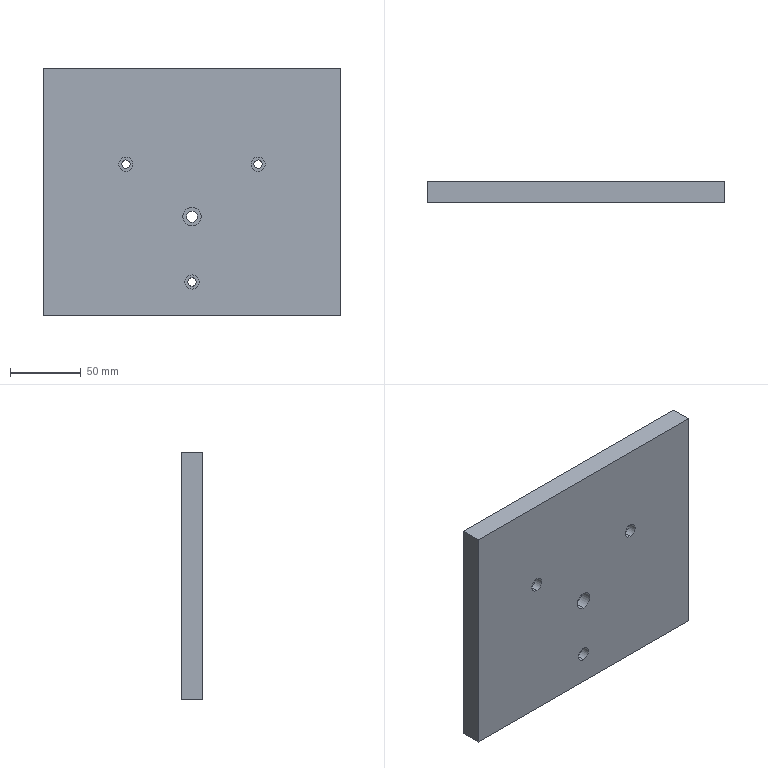Part | SolidWorks | features Cut 4, 3DProfileFeature 2, HoleWzd 2, Extrusion 1 | 1 solid | 46 faces | box 210 x 15 x 175 mm | volume 546137 mm3 | cylinder 26 | cone 10 | plane 10 | commonest cylinder face diameters 5 x10 6 x6 10 x6 8 x2 13 x2
STEP:
#1=CARTESIAN_POINT('',(0.,15.,-21.5));
#2=VERTEX_POINT('',#1);
#3=CARTESIAN_POINT('',(0.,15.,-13.5));
#4=VERTEX_POINT('',#3);
#5=CARTESIAN_POINT('',(0.,15.,-17.5));
#6=DIRECTION('',(0.,1.,0.));
#7=DIRECTION('',(0.,0.,-1.));
#8=AXIS2_PLACEMENT_3D('',#5,#6,#7);
#9=CIRCLE('',#8,4.);
#10=EDGE_CURVE('',#2,#4,#9,.T.);
#11=ORIENTED_EDGE('',*,*,#10,.T.);
#12=CARTESIAN_POINT('',(0.,8.,-13.5));
#13=VERTEX_POINT('',#12);
#14=CARTESIAN_POINT('',(0.,15.001,-13.5));
#15=DIRECTION('',(0.,-1.,0.));
#16=VECTOR('',#15,1000.);
#17=LINE('',#14,#16);
#18=EDGE_CURVE('',#4,#13,#17,.T.);
#19=ORIENTED_EDGE('',*,*,#18,.T.);
#20=CARTESIAN_POINT('',(0.,8.,-21.5));
#21=VERTEX_POINT('',#20);
#22=CARTESIAN_POINT('',(0.,8.,-17.5));
#23=DIRECTION('',(0.,1.,0.));
#24=DIRECTION('',(0.,0.,-1.));
#25=AXIS2_PLACEMENT_3D('',#22,#23,#24);
#26=CIRCLE('',#25,4.);
#27=EDGE_CURVE('',#21,#13,#26,.T.);
#28=ORIENTED_EDGE('',*,*,#27,.F.);
#29=CARTESIAN_POINT('',(0.,15.001,-21.5));
#30=DIRECTION('',(0.,-1.,0.));
#31=VECTOR('',#30,1000.);
#32=LINE('',#29,#31);
#33=EDGE_CURVE('',#2,#21,#32,.T.);
#34=ORIENTED_EDGE('',*,*,#33,.F.);
#35=EDGE_LOOP('',(#11,#19,#28,#34));
#36=FACE_OUTER_BOUND('',#35,.T.);
#37=CARTESIAN_POINT('',(0.,15.001,-17.5));
#38=DIRECTION('',(0.,-1.,0.));
#39=DIRECTION('',(0.,0.,-1.));
#40=AXIS2_PLACEMENT_3D('',#37,#38,#39);
#41=CYLINDRICAL_SURFACE('',#40,4.);
#42=ADVANCED_FACE('',(#36),#41,.F.);
#43=CARTESIAN_POINT('',(0.,8.,-11.));
#44=VERTEX_POINT('',#43);
#45=CARTESIAN_POINT('',(0.,8.,-24.));
#46=VERTEX_POINT('',#45);
#47=CARTESIAN_POINT('',(0.,8.,-17.5));
#48=DIRECTION('',(0.,-1.,0.));
#49=DIRECTION('',(0.,0.,-1.));
#50=AXIS2_PLACEMENT_3D('',#47,#48,#49);
#51=CIRCLE('',#50,6.5);
#52=EDGE_CURVE('',#44,#46,#51,.T.);
#53=ORIENTED_EDGE('',*,*,#52,.F.);
#54=CARTESIAN_POINT('',(0.,0.,-11.));
#55=VERTEX_POINT('',#54);
#56=CARTESIAN_POINT('',(0.,8.,-11.));
#57=DIRECTION('',(0.,-1.,0.));
#58=VECTOR('',#57,1000.);
#59=LINE('',#56,#58);
#60=EDGE_CURVE('',#44,#55,#59,.T.);
#61=ORIENTED_EDGE('',*,*,#60,.T.);
#62=CARTESIAN_POINT('',(0.,0.,-24.));
#63=VERTEX_POINT('',#62);
#64=CARTESIAN_POINT('',(0.,0.,-17.5));
#65=DIRECTION('',(0.,-1.,0.));
#66=DIRECTION('',(0.,0.,-1.));
#67=AXIS2_PLACEMENT_3D('',#64,#65,#66);
#68=CIRCLE('',#67,6.5);
#69=EDGE_CURVE('',#55,#63,#68,.T.);
#70=ORIENTED_EDGE('',*,*,#69,.T.);
#71=CARTESIAN_POINT('',(0.,8.,-24.));
#72=DIRECTION('',(0.,-1.,0.));
#73=VECTOR('',#72,1000.);
#74=LINE('',#71,#73);
#75=EDGE_CURVE('',#46,#63,#74,.T.);
#76=ORIENTED_EDGE('',*,*,#75,.F.);
#77=EDGE_LOOP('',(#53,#61,#70,#76));
#78=FACE_OUTER_BOUND('',#77,.T.);
#79=CARTESIAN_POINT('',(0.,8.,-17.5));
#80=DIRECTION('',(0.,-1.,0.));
#81=DIRECTION('',(0.,0.,-1.));
#82=AXIS2_PLACEMENT_3D('',#79,#80,#81);
#83=CYLINDRICAL_SURFACE('',#82,6.5);
#84=ADVANCED_FACE('',(#78),#83,.F.);
#85=CARTESIAN_POINT('',(82.5,7.5,-72.5));
#86=VERTEX_POINT('',#85);
#87=CARTESIAN_POINT('',(77.5,7.5,-72.5));
#88=VERTEX_POINT('',#87);
#89=CARTESIAN_POINT('',(80.,7.5,-72.5));
#90=DIRECTION('',(0.,0.,-1.));
#91=DIRECTION('',(-1.,0.,0.));
#92=AXIS2_PLACEMENT_3D('',#89,#90,#91);
#93=CIRCLE('',#92,2.5);
#94=EDGE_CURVE('',#86,#88,#93,.T.);
#95=ORIENTED_EDGE('',*,*,#94,.F.);
#96=CARTESIAN_POINT('',(82.5,7.5,-87.5));
#97=VERTEX_POINT('',#96);
#98=CARTESIAN_POINT('',(82.5,7.5,-87.5));
#99=DIRECTION('',(0.,0.,-1.));
#100=VECTOR('',#99,1000.);
#101=LINE('',#98,#100);
#102=EDGE_CURVE('',#86,#97,#101,.T.);
#103=ORIENTED_EDGE('',*,*,#102,.T.);
#104=CARTESIAN_POINT('',(77.5,7.5,-87.5));
#105=VERTEX_POINT('',#104);
#106=CARTESIAN_POINT('',(80.,7.5,-87.5));
#107=DIRECTION('',(0.,0.,-1.));
#108=DIRECTION('',(-1.,0.,0.));
#109=AXIS2_PLACEMENT_3D('',#106,#107,#108);
#110=CIRCLE('',#109,2.5);
#111=EDGE_CURVE('',#97,#105,#110,.T.);
#112=ORIENTED_EDGE('',*,*,#111,.T.);
#113=CARTESIAN_POINT('',(77.5,7.5,-87.5));
#114=DIRECTION('',(0.,0.,-1.));
#115=VECTOR('',#114,1000.);
#116=LINE('',#113,#115);
#117=EDGE_CURVE('',#88,#105,#116,.T.);
#118=ORIENTED_EDGE('',*,*,#117,.F.);
#119=EDGE_LOOP('',(#95,#103,#112,#118));
#120=FACE_OUTER_BOUND('',#119,.T.);
#121=CARTESIAN_POINT('',(80.,7.5,-87.5));
#122=DIRECTION('',(0.,0.,-1.));
#123=DIRECTION('',(-1.,0.,0.));
#124=AXIS2_PLACEMENT_3D('',#121,#122,#123);
#125=CYLINDRICAL_SURFACE('',#124,2.5);
#126=ADVANCED_FACE('',(#120),#125,.F.);
#127=CARTESIAN_POINT('',(80.,7.5,-70.998));
#128=VERTEX_POINT('',#127);
#129=CARTESIAN_POINT('',(77.5,7.5,-72.5));
#130=DIRECTION('',(-0.8572,0.,-0.515));
#131=VECTOR('',#130,1000.);
#132=LINE('',#129,#131);
#133=EDGE_CURVE('',#128,#88,#132,.T.);
#134=ORIENTED_EDGE('',*,*,#133,.F.);
#135=CARTESIAN_POINT('',(82.5,7.5,-72.5));
#136=DIRECTION('',(0.8572,0.,-0.515));
#137=VECTOR('',#136,1000.);
#138=LINE('',#135,#137);
#139=EDGE_CURVE('',#128,#86,#138,.T.);
#140=ORIENTED_EDGE('',*,*,#139,.T.);
#141=ORIENTED_EDGE('',*,*,#94,.T.);
#142=EDGE_LOOP('',(#134,#140,#141));
#143=FACE_OUTER_BOUND('',#142,.T.);
#144=CARTESIAN_POINT('',(80.,7.5,-72.5));
#145=DIRECTION('',(0.,0.,-1.));
#146=DIRECTION('',(-1.,0.,0.));
#147=AXIS2_PLACEMENT_3D('',#144,#145,#146);
#148=CONICAL_SURFACE('',#147,2.5,1.03);
#149=ADVANCED_FACE('',(#143),#148,.F.);
#150=CARTESIAN_POINT('',(2.5,7.5,-72.5));
#151=VERTEX_POINT('',#150);
#152=CARTESIAN_POINT('',(-2.5,7.5,-72.5));
#153=VERTEX_POINT('',#152);
#154=CARTESIAN_POINT('',(0.,7.5,-72.5));
#155=DIRECTION('',(0.,0.,-1.));
#156=DIRECTION('',(-1.,0.,0.));
#157=AXIS2_PLACEMENT_3D('',#154,#155,#156);
#158=CIRCLE('',#157,2.5);
#159=EDGE_CURVE('',#151,#153,#158,.T.);
#160=ORIENTED_EDGE('',*,*,#159,.F.);
#161=CARTESIAN_POINT('',(2.5,7.5,-87.5));
#162=VERTEX_POINT('',#161);
#163=CARTESIAN_POINT('',(2.5,7.5,-87.5));
#164=DIRECTION('',(0.,0.,-1.));
#165=VECTOR('',#164,1000.);
#166=LINE('',#163,#165);
#167=EDGE_CURVE('',#151,#162,#166,.T.);
#168=ORIENTED_EDGE('',*,*,#167,.T.);
#169=CARTESIAN_POINT('',(-2.5,7.5,-87.5));
#170=VERTEX_POINT('',#169);
#171=CARTESIAN_POINT('',(0.,7.5,-87.5));
#172=DIRECTION('',(0.,0.,-1.));
#173=DIRECTION('',(-1.,0.,0.));
#174=AXIS2_PLACEMENT_3D('',#171,#172,#173);
#175=CIRCLE('',#174,2.5);
#176=EDGE_CURVE('',#162,#170,#175,.T.);
#177=ORIENTED_EDGE('',*,*,#176,.T.);
#178=CARTESIAN_POINT('',(-2.5,7.5,-87.5));
#179=DIRECTION('',(0.,0.,-1.));
#180=VECTOR('',#179,1000.);
#181=LINE('',#178,#180);
#182=EDGE_CURVE('',#153,#170,#181,.T.);
#183=ORIENTED_EDGE('',*,*,#182,.F.);
#184=EDGE_LOOP('',(#160,#168,#177,#183));
#185=FACE_OUTER_BOUND('',#184,.T.);
#186=CARTESIAN_POINT('',(0.,7.5,-87.5));
#187=DIRECTION('',(0.,0.,-1.));
#188=DIRECTION('',(-1.,0.,0.));
#189=AXIS2_PLACEMENT_3D('',#186,#187,#188);
#190=CYLINDRICAL_SURFACE('',#189,2.5);
#191=ADVANCED_FACE('',(#185),#190,.F.);
#192=CARTESIAN_POINT('',(0.,7.5,-70.998));
#193=VERTEX_POINT('',#192);
#194=CARTESIAN_POINT('',(-2.5,7.5,-72.5));
#195=DIRECTION('',(-0.8572,0.,-0.515));
#196=VECTOR('',#195,1000.);
#197=LINE('',#194,#196);
#198=EDGE_CURVE('',#193,#153,#197,.T.);
#199=ORIENTED_EDGE('',*,*,#198,.F.);
#200=CARTESIAN_POINT('',(2.5,7.5,-72.5));
#201=DIRECTION('',(0.8572,0.,-0.515));
#202=VECTOR('',#201,1000.);
#203=LINE('',#200,#202);
#204=EDGE_CURVE('',#193,#151,#203,.T.);
#205=ORIENTED_EDGE('',*,*,#204,.T.);
#206=ORIENTED_EDGE('',*,*,#159,.T.);
#207=EDGE_LOOP('',(#199,#205,#206));
#208=FACE_OUTER_BOUND('',#207,.T.);
#209=CARTESIAN_POINT('',(0.,7.5,-72.5));
#210=DIRECTION('',(0.,0.,-1.));
#211=DIRECTION('',(-1.,0.,0.));
#212=AXIS2_PLACEMENT_3D('',#209,#210,#211);
#213=CONICAL_SURFACE('',#212,2.5,1.03);
#214=ADVANCED_FACE('',(#208),#213,.F.);
#215=CARTESIAN_POINT('',(-77.5,7.5,-72.5));
#216=VERTEX_POINT('',#215);
#217=CARTESIAN_POINT('',(-82.5,7.5,-72.5));
#218=VERTEX_POINT('',#217);
#219=CARTESIAN_POINT('',(-80.,7.5,-72.5));
#220=DIRECTION('',(0.,0.,-1.));
#221=DIRECTION('',(-1.,0.,0.));
#222=AXIS2_PLACEMENT_3D('',#219,#220,#221);
#223=CIRCLE('',#222,2.5);
#224=EDGE_CURVE('',#216,#218,#223,.T.);
#225=ORIENTED_EDGE('',*,*,#224,.F.);
#226=CARTESIAN_POINT('',(-77.5,7.5,-87.5));
#227=VERTEX_POINT('',#226);
#228=CARTESIAN_POINT('',(-77.5,7.5,-87.5));
#229=DIRECTION('',(0.,0.,-1.));
#230=VECTOR('',#229,1000.);
#231=LINE('',#228,#230);
#232=EDGE_CURVE('',#216,#227,#231,.T.);
#233=ORIENTED_EDGE('',*,*,#232,.T.);
#234=CARTESIAN_POINT('',(-82.5,7.5,-87.5));
#235=VERTEX_POINT('',#234);
#236=CARTESIAN_POINT('',(-80.,7.5,-87.5));
#237=DIRECTION('',(0.,0.,-1.));
#238=DIRECTION('',(-1.,0.,0.));
#239=AXIS2_PLACEMENT_3D('',#236,#237,#238);
#240=CIRCLE('',#239,2.5);
#241=EDGE_CURVE('',#227,#235,#240,.T.);
#242=ORIENTED_EDGE('',*,*,#241,.T.);
#243=CARTESIAN_POINT('',(-82.5,7.5,-87.5));
#244=DIRECTION('',(0.,0.,-1.));
#245=VECTOR('',#244,1000.);
#246=LINE('',#243,#245);
#247=EDGE_CURVE('',#218,#235,#246,.T.);
#248=ORIENTED_EDGE('',*,*,#247,.F.);
#249=EDGE_LOOP('',(#225,#233,#242,#248));
#250=FACE_OUTER_BOUND('',#249,.T.);
#251=CARTESIAN_POINT('',(-80.,7.5,-87.5));
#252=DIRECTION('',(0.,0.,-1.));
#253=DIRECTION('',(-1.,0.,0.));
#254=AXIS2_PLACEMENT_3D('',#251,#252,#253);
#255=CYLINDRICAL_SURFACE('',#254,2.5);
#256=ADVANCED_FACE('',(#250),#255,.F.);
#257=CARTESIAN_POINT('',(-80.,7.5,-70.998));
#258=VERTEX_POINT('',#257);
#259=CARTESIAN_POINT('',(-82.5,7.5,-72.5));
#260=DIRECTION('',(-0.8572,0.,-0.515));
#261=VECTOR('',#260,1000.);
#262=LINE('',#259,#261);
#263=EDGE_CURVE('',#258,#218,#262,.T.);
#264=ORIENTED_EDGE('',*,*,#263,.F.);
#265=CARTESIAN_POINT('',(-77.5,7.5,-72.5));
#266=DIRECTION('',(0.8572,0.,-0.515));
#267=VECTOR('',#266,1000.);
#268=LINE('',#265,#267);
#269=EDGE_CURVE('',#258,#216,#268,.T.);
#270=ORIENTED_EDGE('',*,*,#269,.T.);
#271=ORIENTED_EDGE('',*,*,#224,.T.);
#272=EDGE_LOOP('',(#264,#270,#271));
#273=FACE_OUTER_BOUND('',#272,.T.);
#274=CARTESIAN_POINT('',(-80.,7.5,-72.5));
#275=DIRECTION('',(0.,0.,-1.));
#276=DIRECTION('',(-1.,0.,0.));
#277=AXIS2_PLACEMENT_3D('',#274,#275,#276);
#278=CONICAL_SURFACE('',#277,2.5,1.03);
#279=ADVANCED_FACE('',(#273),#278,.F.);
#280=CARTESIAN_POINT('',(90.,7.5,-13.5));
#281=VERTEX_POINT('',#280);
#282=CARTESIAN_POINT('',(90.,7.5,-18.5));
#283=VERTEX_POINT('',#282);
#284=CARTESIAN_POINT('',(90.,7.5,-16.));
#285=DIRECTION('',(1.,0.,0.));
#286=DIRECTION('',(0.,0.,-1.));
#287=AXIS2_PLACEMENT_3D('',#284,#285,#286);
#288=CIRCLE('',#287,2.5);
#289=EDGE_CURVE('',#281,#283,#288,.T.);
#290=ORIENTED_EDGE('',*,*,#289,.F.);
#291=CARTESIAN_POINT('',(105.,7.5,-13.5));
#292=VERTEX_POINT('',#291);
#293=CARTESIAN_POINT('',(105.,7.5,-13.5));
#294=DIRECTION('',(1.,0.,0.));
#295=VECTOR('',#294,1000.);
#296=LINE('',#293,#295);
#297=EDGE_CURVE('',#281,#292,#296,.T.);
#298=ORIENTED_EDGE('',*,*,#297,.T.);
#299=CARTESIAN_POINT('',(105.,7.5,-18.5));
#300=VERTEX_POINT('',#299);
#301=CARTESIAN_POINT('',(105.,7.5,-16.));
#302=DIRECTION('',(1.,0.,0.));
#303=DIRECTION('',(0.,0.,-1.));
#304=AXIS2_PLACEMENT_3D('',#301,#302,#303);
#305=CIRCLE('',#304,2.5);
#306=EDGE_CURVE('',#292,#300,#305,.T.);
#307=ORIENTED_EDGE('',*,*,#306,.T.);
#308=CARTESIAN_POINT('',(105.,7.5,-18.5));
#309=DIRECTION('',(1.,0.,0.));
#310=VECTOR('',#309,1000.);
#311=LINE('',#308,#310);
#312=EDGE_CURVE('',#283,#300,#311,.T.);
#313=ORIENTED_EDGE('',*,*,#312,.F.);
#314=EDGE_LOOP('',(#290,#298,#307,#313));
#315=FACE_OUTER_BOUND('',#314,.T.);
#316=CARTESIAN_POINT('',(105.,7.5,-16.));
#317=DIRECTION('',(1.,0.,0.));
#318=DIRECTION('',(0.,0.,-1.));
#319=AXIS2_PLACEMENT_3D('',#316,#317,#318);
#320=CYLINDRICAL_SURFACE('',#319,2.5);
#321=ADVANCED_FACE('',(#315),#320,.F.);
#322=CARTESIAN_POINT('',(88.498,7.5,-16.));
#323=VERTEX_POINT('',#322);
#324=CARTESIAN_POINT('',(90.,7.5,-18.5));
#325=DIRECTION('',(0.515,0.,-0.8572));
#326=VECTOR('',#325,1000.);
#327=LINE('',#324,#326);
#328=EDGE_CURVE('',#323,#283,#327,.T.);
#329=ORIENTED_EDGE('',*,*,#328,.F.);
#330=CARTESIAN_POINT('',(90.,7.5,-13.5));
#331=DIRECTION('',(0.515,0.,0.8572));
#332=VECTOR('',#331,1000.);
#333=LINE('',#330,#332);
#334=EDGE_CURVE('',#323,#281,#333,.T.);
#335=ORIENTED_EDGE('',*,*,#334,.T.);
#336=ORIENTED_EDGE('',*,*,#289,.T.);
#337=EDGE_LOOP('',(#329,#335,#336));
#338=FACE_OUTER_BOUND('',#337,.T.);
#339=CARTESIAN_POINT('',(90.,7.5,-16.));
#340=DIRECTION('',(1.,0.,0.));
#341=DIRECTION('',(0.,0.,-1.));
#342=AXIS2_PLACEMENT_3D('',#339,#340,#341);
#343=CONICAL_SURFACE('',#342,2.5,1.03);
#344=ADVANCED_FACE('',(#338),#343,.F.);
#345=CARTESIAN_POINT('',(90.,7.5,64.5));
#346=VERTEX_POINT('',#345);
#347=CARTESIAN_POINT('',(90.,7.5,59.5));
#348=VERTEX_POINT('',#347);
#349=CARTESIAN_POINT('',(90.,7.5,62.));
#350=DIRECTION('',(1.,0.,0.));
#351=DIRECTION('',(0.,0.,-1.));
#352=AXIS2_PLACEMENT_3D('',#349,#350,#351);
#353=CIRCLE('',#352,2.5);
#354=EDGE_CURVE('',#346,#348,#353,.T.);
#355=ORIENTED_EDGE('',*,*,#354,.F.);
#356=CARTESIAN_POINT('',(105.,7.5,64.5));
#357=VERTEX_POINT('',#356);
#358=CARTESIAN_POINT('',(105.,7.5,64.5));
#359=DIRECTION('',(1.,0.,0.));
#360=VECTOR('',#359,1000.);
#361=LINE('',#358,#360);
#362=EDGE_CURVE('',#346,#357,#361,.T.);
#363=ORIENTED_EDGE('',*,*,#362,.T.);
#364=CARTESIAN_POINT('',(105.,7.5,59.5));
#365=VERTEX_POINT('',#364);
#366=CARTESIAN_POINT('',(105.,7.5,62.));
#367=DIRECTION('',(1.,0.,0.));
#368=DIRECTION('',(0.,0.,-1.));
#369=AXIS2_PLACEMENT_3D('',#366,#367,#368);
#370=CIRCLE('',#369,2.5);
#371=EDGE_CURVE('',#357,#365,#370,.T.);
#372=ORIENTED_EDGE('',*,*,#371,.T.);
#373=CARTESIAN_POINT('',(105.,7.5,59.5));
#374=DIRECTION('',(1.,0.,0.));
#375=VECTOR('',#374,1000.);
#376=LINE('',#373,#375);
#377=EDGE_CURVE('',#348,#365,#376,.T.);
#378=ORIENTED_EDGE('',*,*,#377,.F.);
#379=EDGE_LOOP('',(#355,#363,#372,#378));
#380=FACE_OUTER_BOUND('',#379,.T.);
#381=CARTESIAN_POINT('',(105.,7.5,62.));
#382=DIRECTION('',(1.,0.,0.));
#383=DIRECTION('',(0.,0.,-1.));
#384=AXIS2_PLACEMENT_3D('',#381,#382,#383);
#385=CYLINDRICAL_SURFACE('',#384,2.5);
#386=ADVANCED_FACE('',(#380),#385,.F.);
#387=CARTESIAN_POINT('',(88.498,7.5,62.));
#388=VERTEX_POINT('',#387);
#389=CARTESIAN_POINT('',(90.,7.5,59.5));
#390=DIRECTION('',(0.515,0.,-0.8572));
#391=VECTOR('',#390,1000.);
#392=LINE('',#389,#391);
#393=EDGE_CURVE('',#388,#348,#392,.T.);
#394=ORIENTED_EDGE('',*,*,#393,.F.);
#395=CARTESIAN_POINT('',(90.,7.5,64.5));
#396=DIRECTION('',(0.515,0.,0.8572));
#397=VECTOR('',#396,1000.);
#398=LINE('',#395,#397);
#399=EDGE_CURVE('',#388,#346,#398,.T.);
#400=ORIENTED_EDGE('',*,*,#399,.T.);
#401=ORIENTED_EDGE('',*,*,#354,.T.);
#402=EDGE_LOOP('',(#394,#400,#401));
#403=FACE_OUTER_BOUND('',#402,.T.);
#404=CARTESIAN_POINT('',(90.,7.5,62.));
#405=DIRECTION('',(1.,0.,0.));
#406=DIRECTION('',(0.,0.,-1.));
#407=AXIS2_PLACEMENT_3D('',#404,#405,#406);
#408=CONICAL_SURFACE('',#407,2.5,1.03);
#409=ADVANCED_FACE('',(#403),#408,.F.);
#410=CARTESIAN_POINT('',(0.,15.,-66.627));
#411=VERTEX_POINT('',#410);
#412=CARTESIAN_POINT('',(0.,15.,-60.627));
#413=VERTEX_POINT('',#412);
#414=CARTESIAN_POINT('',(0.,15.,-63.627));
#415=DIRECTION('',(0.,1.,0.));
#416=DIRECTION('',(0.,0.,-1.));
#417=AXIS2_PLACEMENT_3D('',#414,#415,#416);
#418=CIRCLE('',#417,3.);
#419=EDGE_CURVE('',#411,#413,#418,.T.);
#420=ORIENTED_EDGE('',*,*,#419,.T.);
#421=CARTESIAN_POINT('',(0.,6.,-60.627));
#422=VERTEX_POINT('',#421);
#423=CARTESIAN_POINT('',(0.,15.001,-60.627));
#424=DIRECTION('',(0.,-1.,0.));
#425=VECTOR('',#424,1000.);
#426=LINE('',#423,#425);
#427=EDGE_CURVE('',#413,#422,#426,.T.);
#428=ORIENTED_EDGE('',*,*,#427,.T.);
#429=CARTESIAN_POINT('',(0.,6.,-66.627));
#430=VERTEX_POINT('',#429);
#431=CARTESIAN_POINT('',(0.,6.,-63.627));
#432=DIRECTION('',(0.,1.,0.));
#433=DIRECTION('',(0.,0.,-1.));
#434=AXIS2_PLACEMENT_3D('',#431,#432,#433);
#435=CIRCLE('',#434,3.);
#436=EDGE_CURVE('',#430,#422,#435,.T.);
#437=ORIENTED_EDGE('',*,*,#436,.F.);
#438=CARTESIAN_POINT('',(0.,15.001,-66.627));
#439=DIRECTION('',(0.,-1.,0.));
#440=VECTOR('',#439,1000.);
#441=LINE('',#438,#440);
#442=EDGE_CURVE('',#411,#430,#441,.T.);
#443=ORIENTED_EDGE('',*,*,#442,.F.);
#444=EDGE_LOOP('',(#420,#428,#437,#443));
#445=FACE_OUTER_BOUND('',#444,.T.);
#446=CARTESIAN_POINT('',(0.,15.001,-63.627));
#447=DIRECTION('',(0.,-1.,0.));
#448=DIRECTION('',(0.,0.,-1.));
#449=AXIS2_PLACEMENT_3D('',#446,#447,#448);
#450=CYLINDRICAL_SURFACE('',#449,3.);
#451=ADVANCED_FACE('',(#445),#450,.F.);
#452=CARTESIAN_POINT('',(46.688,15.,16.638));
#453=VERTEX_POINT('',#452);
#454=CARTESIAN_POINT('',(46.688,15.,22.638));
#455=VERTEX_POINT('',#454);
#456=CARTESIAN_POINT('',(46.688,15.,19.638));
#457=DIRECTION('',(0.,1.,0.));
#458=DIRECTION('',(0.,0.,-1.));
#459=AXIS2_PLACEMENT_3D('',#456,#457,#458);
#460=CIRCLE('',#459,3.);
#461=EDGE_CURVE('',#453,#455,#460,.T.);
#462=ORIENTED_EDGE('',*,*,#461,.T.);
#463=CARTESIAN_POINT('',(46.688,6.,22.638));
#464=VERTEX_POINT('',#463);
#465=CARTESIAN_POINT('',(46.688,15.001,22.638));
#466=DIRECTION('',(0.,-1.,0.));
#467=VECTOR('',#466,1000.);
#468=LINE('',#465,#467);
#469=EDGE_CURVE('',#455,#464,#468,.T.);
#470=ORIENTED_EDGE('',*,*,#469,.T.);
#471=CARTESIAN_POINT('',(46.688,6.,16.638));
#472=VERTEX_POINT('',#471);
#473=CARTESIAN_POINT('',(46.688,6.,19.638));
#474=DIRECTION('',(0.,1.,0.));
#475=DIRECTION('',(0.,0.,-1.));
#476=AXIS2_PLACEMENT_3D('',#473,#474,#475);
#477=CIRCLE('',#476,3.);
#478=EDGE_CURVE('',#472,#464,#477,.T.);
#479=ORIENTED_EDGE('',*,*,#478,.F.);
#480=CARTESIAN_POINT('',(46.688,15.001,16.638));
#481=DIRECTION('',(0.,-1.,0.));
#482=VECTOR('',#481,1000.);
#483=LINE('',#480,#482);
#484=EDGE_CURVE('',#453,#472,#483,.T.);
#485=ORIENTED_EDGE('',*,*,#484,.F.);
#486=EDGE_LOOP('',(#462,#470,#479,#485));
#487=FACE_OUTER_BOUND('',#486,.T.);
#488=CARTESIAN_POINT('',(46.688,15.001,19.638));
#489=DIRECTION('',(0.,-1.,0.));
#490=DIRECTION('',(0.,0.,-1.));
#491=AXIS2_PLACEMENT_3D('',#488,#489,#490);
#492=CYLINDRICAL_SURFACE('',#491,3.);
#493=ADVANCED_FACE('',(#487),#492,.F.);
#494=CARTESIAN_POINT('',(-46.688,15.,16.638));
#495=VERTEX_POINT('',#494);
#496=CARTESIAN_POINT('',(-46.688,15.,22.638));
#497=VERTEX_POINT('',#496);
#498=CARTESIAN_POINT('',(-46.688,15.,19.638));
#499=DIRECTION('',(0.,1.,0.));
#500=DIRECTION('',(0.,0.,-1.));
#501=AXIS2_PLACEMENT_3D('',#498,#499,#500);
#502=CIRCLE('',#501,3.);
#503=EDGE_CURVE('',#495,#497,#502,.T.);
#504=ORIENTED_EDGE('',*,*,#503,.T.);
#505=CARTESIAN_POINT('',(-46.688,6.,22.638));
#506=VERTEX_POINT('',#505);
#507=CARTESIAN_POINT('',(-46.688,15.001,22.638));
#508=DIRECTION('',(0.,-1.,0.));
#509=VECTOR('',#508,1000.);
#510=LINE('',#507,#509);
#511=EDGE_CURVE('',#497,#506,#510,.T.);
#512=ORIENTED_EDGE('',*,*,#511,.T.);
#513=CARTESIAN_POINT('',(-46.688,6.,16.638));
#514=VERTEX_POINT('',#513);
#515=CARTESIAN_POINT('',(-46.688,6.,19.638));
#516=DIRECTION('',(0.,1.,0.));
#517=DIRECTION('',(0.,0.,-1.));
#518=AXIS2_PLACEMENT_3D('',#515,#516,#517);
#519=CIRCLE('',#518,3.);
#520=EDGE_CURVE('',#514,#506,#519,.T.);
#521=ORIENTED_EDGE('',*,*,#520,.F.);
#522=CARTESIAN_POINT('',(-46.688,15.001,16.638));
#523=DIRECTION('',(0.,-1.,0.));
#524=VECTOR('',#523,1000.);
#525=LINE('',#522,#524);
#526=EDGE_CURVE('',#495,#514,#525,.T.);
#527=ORIENTED_EDGE('',*,*,#526,.F.);
#528=EDGE_LOOP('',(#504,#512,#521,#527));
#529=FACE_OUTER_BOUND('',#528,.T.);
#530=CARTESIAN_POINT('',(-46.688,15.001,19.638));
#531=DIRECTION('',(0.,-1.,0.));
#532=DIRECTION('',(0.,0.,-1.));
#533=AXIS2_PLACEMENT_3D('',#530,#531,#532);
#534=CYLINDRICAL_SURFACE('',#533,3.);
#535=ADVANCED_FACE('',(#529),#534,.F.);
#536=CARTESIAN_POINT('',(0.,6.,-58.627));
#537=VERTEX_POINT('',#536);
#538=CARTESIAN_POINT('',(0.,6.,-68.627));
#539=VERTEX_POINT('',#538);
#540=CARTESIAN_POINT('',(0.,6.,-63.627));
#541=DIRECTION('',(0.,-1.,0.));
#542=DIRECTION('',(0.,0.,-1.));
#543=AXIS2_PLACEMENT_3D('',#540,#541,#542);
#544=CIRCLE('',#543,5.);
#545=EDGE_CURVE('',#537,#539,#544,.T.);
#546=ORIENTED_EDGE('',*,*,#545,.F.);
#547=CARTESIAN_POINT('',(0.,0.,-58.627));
#548=VERTEX_POINT('',#547);
#549=CARTESIAN_POINT('',(0.,6.,-58.627));
#550=DIRECTION('',(0.,-1.,0.));
#551=VECTOR('',#550,1000.);
#552=LINE('',#549,#551);
#553=EDGE_CURVE('',#537,#548,#552,.T.);
#554=ORIENTED_EDGE('',*,*,#553,.T.);
#555=CARTESIAN_POINT('',(0.,0.,-68.627));
#556=VERTEX_POINT('',#555);
#557=CARTESIAN_POINT('',(0.,0.,-63.627));
#558=DIRECTION('',(0.,-1.,0.));
#559=DIRECTION('',(0.,0.,-1.));
#560=AXIS2_PLACEMENT_3D('',#557,#558,#559);
#561=CIRCLE('',#560,5.);
#562=EDGE_CURVE('',#548,#556,#561,.T.);
#563=ORIENTED_EDGE('',*,*,#562,.T.);
#564=CARTESIAN_POINT('',(0.,6.,-68.627));
#565=DIRECTION('',(0.,-1.,0.));
#566=VECTOR('',#565,1000.);
#567=LINE('',#564,#566);
#568=EDGE_CURVE('',#539,#556,#567,.T.);
#569=ORIENTED_EDGE('',*,*,#568,.F.);
#570=EDGE_LOOP('',(#546,#554,#563,#569));
#571=FACE_OUTER_BOUND('',#570,.T.);
#572=CARTESIAN_POINT('',(0.,6.,-63.627));
#573=DIRECTION('',(0.,-1.,0.));
#574=DIRECTION('',(0.,0.,-1.));
#575=AXIS2_PLACEMENT_3D('',#572,#573,#574);
#576=CYLINDRICAL_SURFACE('',#575,5.);
#577=ADVANCED_FACE('',(#571),#576,.F.);
#578=CARTESIAN_POINT('',(46.688,6.,24.638));
#579=VERTEX_POINT('',#578);
#580=CARTESIAN_POINT('',(46.688,6.,14.638));
#581=VERTEX_POINT('',#580);
#582=CARTESIAN_POINT('',(46.688,6.,19.638));
#583=DIRECTION('',(0.,-1.,0.));
#584=DIRECTION('',(0.,0.,-1.));
#585=AXIS2_PLACEMENT_3D('',#582,#583,#584);
#586=CIRCLE('',#585,5.);
#587=EDGE_CURVE('',#579,#581,#586,.T.);
#588=ORIENTED_EDGE('',*,*,#587,.F.);
#589=CARTESIAN_POINT('',(46.688,0.,24.638));
#590=VERTEX_POINT('',#589);
#591=CARTESIAN_POINT('',(46.688,6.,24.638));
#592=DIRECTION('',(0.,-1.,0.));
#593=VECTOR('',#592,1000.);
#594=LINE('',#591,#593);
#595=EDGE_CURVE('',#579,#590,#594,.T.);
#596=ORIENTED_EDGE('',*,*,#595,.T.);
#597=CARTESIAN_POINT('',(46.688,0.,14.638));
#598=VERTEX_POINT('',#597);
#599=CARTESIAN_POINT('',(46.688,0.,19.638));
#600=DIRECTION('',(0.,-1.,0.));
#601=DIRECTION('',(0.,0.,-1.));
#602=AXIS2_PLACEMENT_3D('',#599,#600,#601);
#603=CIRCLE('',#602,5.);
#604=EDGE_CURVE('',#590,#598,#603,.T.);
#605=ORIENTED_EDGE('',*,*,#604,.T.);
#606=CARTESIAN_POINT('',(46.688,6.,14.638));
#607=DIRECTION('',(0.,-1.,0.));
#608=VECTOR('',#607,1000.);
#609=LINE('',#606,#608);
#610=EDGE_CURVE('',#581,#598,#609,.T.);
#611=ORIENTED_EDGE('',*,*,#610,.F.);
#612=EDGE_LOOP('',(#588,#596,#605,#611));
#613=FACE_OUTER_BOUND('',#612,.T.);
#614=CARTESIAN_POINT('',(46.688,6.,19.638));
#615=DIRECTION('',(0.,-1.,0.));
#616=DIRECTION('',(0.,0.,-1.));
#617=AXIS2_PLACEMENT_3D('',#614,#615,#616);
#618=CYLINDRICAL_SURFACE('',#617,5.);
#619=ADVANCED_FACE('',(#613),#618,.F.);
#620=CARTESIAN_POINT('',(-46.688,6.,24.638));
#621=VERTEX_POINT('',#620);
#622=CARTESIAN_POINT('',(-46.688,6.,14.638));
#623=VERTEX_POINT('',#622);
#624=CARTESIAN_POINT('',(-46.688,6.,19.638));
#625=DIRECTION('',(0.,-1.,0.));
#626=DIRECTION('',(0.,0.,-1.));
#627=AXIS2_PLACEMENT_3D('',#624,#625,#626);
#628=CIRCLE('',#627,5.);
#629=EDGE_CURVE('',#621,#623,#628,.T.);
#630=ORIENTED_EDGE('',*,*,#629,.F.);
#631=CARTESIAN_POINT('',(-46.688,0.,24.638));
#632=VERTEX_POINT('',#631);
#633=CARTESIAN_POINT('',(-46.688,6.,24.638));
#634=DIRECTION('',(0.,-1.,0.));
#635=VECTOR('',#634,1000.);
#636=LINE('',#633,#635);
#637=EDGE_CURVE('',#621,#632,#636,.T.);
#638=ORIENTED_EDGE('',*,*,#637,.T.);
#639=CARTESIAN_POINT('',(-46.688,0.,14.638));
#640=VERTEX_POINT('',#639);
#641=CARTESIAN_POINT('',(-46.688,0.,19.638));
#642=DIRECTION('',(0.,-1.,0.));
#643=DIRECTION('',(0.,0.,-1.));
#644=AXIS2_PLACEMENT_3D('',#641,#642,#643);
#645=CIRCLE('',#644,5.);
#646=EDGE_CURVE('',#632,#640,#645,.T.);
#647=ORIENTED_EDGE('',*,*,#646,.T.);
#648=CARTESIAN_POINT('',(-46.688,6.,14.638));
#649=DIRECTION('',(0.,-1.,0.));
#650=VECTOR('',#649,1000.);
#651=LINE('',#648,#650);
#652=EDGE_CURVE('',#623,#640,#651,.T.);
#653=ORIENTED_EDGE('',*,*,#652,.F.);
#654=EDGE_LOOP('',(#630,#638,#647,#653));
#655=FACE_OUTER_BOUND('',#654,.T.);
#656=CARTESIAN_POINT('',(-46.688,6.,19.638));
#657=DIRECTION('',(0.,-1.,0.));
#658=DIRECTION('',(0.,0.,-1.));
#659=AXIS2_PLACEMENT_3D('',#656,#657,#658);
#660=CYLINDRICAL_SURFACE('',#659,5.);
#661=ADVANCED_FACE('',(#655),#660,.F.);
#662=CARTESIAN_POINT('',(105.,7.5,-16.));
#663=DIRECTION('',(1.,0.,0.));
#664=DIRECTION('',(0.,0.,-1.));
#665=AXIS2_PLACEMENT_3D('',#662,#663,#664);
#666=CIRCLE('',#665,2.5);
#667=EDGE_CURVE('',#300,#292,#666,.T.);
#668=ORIENTED_EDGE('',*,*,#667,.F.);
#669=ORIENTED_EDGE('',*,*,#306,.F.);
#670=EDGE_LOOP('',(#668,#669));
#671=FACE_BOUND('',#670,.T.);
#672=CARTESIAN_POINT('',(105.,7.5,62.));
#673=DIRECTION('',(1.,0.,0.));
#674=DIRECTION('',(0.,0.,-1.));
#675=AXIS2_PLACEMENT_3D('',#672,#673,#674);
#676=CIRCLE('',#675,2.5);
#677=EDGE_CURVE('',#365,#357,#676,.T.);
#678=ORIENTED_EDGE('',*,*,#677,.F.);
#679=ORIENTED_EDGE('',*,*,#371,.F.);
#680=EDGE_LOOP('',(#678,#679));
#681=FACE_BOUND('',#680,.T.);
#682=CARTESIAN_POINT('',(105.,0.,87.5));
#683=VERTEX_POINT('',#682);
#684=CARTESIAN_POINT('',(105.,0.,-87.5));
#685=VERTEX_POINT('',#684);
#686=CARTESIAN_POINT('',(105.,0.,87.5));
#687=DIRECTION('',(0.,0.,-1.));
#688=VECTOR('',#687,1000.);
#689=LINE('',#686,#688);
#690=EDGE_CURVE('',#683,#685,#689,.T.);
#691=ORIENTED_EDGE('',*,*,#690,.T.);
#692=CARTESIAN_POINT('',(105.,15.,-87.5));
#693=VERTEX_POINT('',#692);
#694=CARTESIAN_POINT('',(105.,15.,-87.5));
#695=DIRECTION('',(0.,-1.,0.));
#696=VECTOR('',#695,1000.);
#697=LINE('',#694,#696);
#698=EDGE_CURVE('',#693,#685,#697,.T.);
#699=ORIENTED_EDGE('',*,*,#698,.F.);
#700=CARTESIAN_POINT('',(105.,15.,87.5));
#701=VERTEX_POINT('',#700);
#702=CARTESIAN_POINT('',(105.,15.,87.5));
#703=DIRECTION('',(0.,0.,-1.));
#704=VECTOR('',#703,1000.);
#705=LINE('',#702,#704);
#706=EDGE_CURVE('',#701,#693,#705,.T.);
#707=ORIENTED_EDGE('',*,*,#706,.F.);
#708=CARTESIAN_POINT('',(105.,15.,87.5));
#709=DIRECTION('',(0.,-1.,0.));
#710=VECTOR('',#709,1000.);
#711=LINE('',#708,#710);
#712=EDGE_CURVE('',#701,#683,#711,.T.);
#713=ORIENTED_EDGE('',*,*,#712,.T.);
#714=EDGE_LOOP('',(#691,#699,#707,#713));
#715=FACE_OUTER_BOUND('',#714,.T.);
#716=CARTESIAN_POINT('',(105.,15.,87.5));
#717=DIRECTION('',(-1.,0.,0.));
#718=DIRECTION('',(0.,0.,1.));
#719=AXIS2_PLACEMENT_3D('',#716,#717,#718);
#720=PLANE('',#719);
#721=ADVANCED_FACE('',(#671,#681,#715),#720,.F.);
#722=CARTESIAN_POINT('',(80.,7.5,-87.5));
#723=DIRECTION('',(0.,0.,-1.));
#724=DIRECTION('',(-1.,0.,0.));
#725=AXIS2_PLACEMENT_3D('',#722,#723,#724);
#726=CIRCLE('',#725,2.5);
#727=EDGE_CURVE('',#105,#97,#726,.T.);
#728=ORIENTED_EDGE('',*,*,#727,.F.);
#729=ORIENTED_EDGE('',*,*,#111,.F.);
#730=EDGE_LOOP('',(#728,#729));
#731=FACE_BOUND('',#730,.T.);
#732=CARTESIAN_POINT('',(0.,7.5,-87.5));
#733=DIRECTION('',(0.,0.,-1.));
#734=DIRECTION('',(-1.,0.,0.));
#735=AXIS2_PLACEMENT_3D('',#732,#733,#734);
#736=CIRCLE('',#735,2.5);
#737=EDGE_CURVE('',#170,#162,#736,.T.);
#738=ORIENTED_EDGE('',*,*,#737,.F.);
#739=ORIENTED_EDGE('',*,*,#176,.F.);
#740=EDGE_LOOP('',(#738,#739));
#741=FACE_BOUND('',#740,.T.);
#742=CARTESIAN_POINT('',(-80.,7.5,-87.5));
#743=DIRECTION('',(0.,0.,-1.));
#744=DIRECTION('',(-1.,0.,0.));
#745=AXIS2_PLACEMENT_3D('',#742,#743,#744);
#746=CIRCLE('',#745,2.5);
#747=EDGE_CURVE('',#235,#227,#746,.T.);
#748=ORIENTED_EDGE('',*,*,#747,.F.);
#749=ORIENTED_EDGE('',*,*,#241,.F.);
#750=EDGE_LOOP('',(#748,#749));
#751=FACE_BOUND('',#750,.T.);
#752=CARTESIAN_POINT('',(-105.,0.,-87.5));
#753=VERTEX_POINT('',#752);
#754=CARTESIAN_POINT('',(-105.,0.,-87.5));
#755=DIRECTION('',(-1.,0.,0.));
#756=VECTOR('',#755,1000.);
#757=LINE('',#754,#756);
#758=EDGE_CURVE('',#685,#753,#757,.T.);
#759=ORIENTED_EDGE('',*,*,#758,.T.);
#760=CARTESIAN_POINT('',(-105.,15.,-87.5));
#761=VERTEX_POINT('',#760);
#762=CARTESIAN_POINT('',(-105.,15.,-87.5));
#763=DIRECTION('',(0.,-1.,0.));
#764=VECTOR('',#763,1000.);
#765=LINE('',#762,#764);
#766=EDGE_CURVE('',#761,#753,#765,.T.);
#767=ORIENTED_EDGE('',*,*,#766,.F.);
#768=CARTESIAN_POINT('',(-105.,15.,-87.5));
#769=DIRECTION('',(-1.,0.,0.));
#770=VECTOR('',#769,1000.);
#771=LINE('',#768,#770);
#772=EDGE_CURVE('',#693,#761,#771,.T.);
#773=ORIENTED_EDGE('',*,*,#772,.F.);
#774=ORIENTED_EDGE('',*,*,#698,.T.);
#775=EDGE_LOOP('',(#759,#767,#773,#774));
#776=FACE_OUTER_BOUND('',#775,.T.);
#777=CARTESIAN_POINT('',(-105.,15.,-87.5));
#778=DIRECTION('',(0.,0.,1.));
#779=DIRECTION('',(1.,0.,0.));
#780=AXIS2_PLACEMENT_3D('',#777,#778,#779);
#781=PLANE('',#780);
#782=ADVANCED_FACE('',(#731,#741,#751,#776),#781,.F.);
#783=CARTESIAN_POINT('',(-105.,0.,87.5));
#784=VERTEX_POINT('',#783);
#785=CARTESIAN_POINT('',(-105.,0.,87.5));
#786=DIRECTION('',(0.,0.,1.));
#787=VECTOR('',#786,1000.);
#788=LINE('',#785,#787);
#789=EDGE_CURVE('',#753,#784,#788,.T.);
#790=ORIENTED_EDGE('',*,*,#789,.T.);
#791=CARTESIAN_POINT('',(-105.,15.,87.5));
#792=VERTEX_POINT('',#791);
#793=CARTESIAN_POINT('',(-105.,15.,87.5));
#794=DIRECTION('',(0.,-1.,0.));
#795=VECTOR('',#794,1000.);
#796=LINE('',#793,#795);
#797=EDGE_CURVE('',#792,#784,#796,.T.);
#798=ORIENTED_EDGE('',*,*,#797,.F.);
#799=CARTESIAN_POINT('',(-105.,15.,87.5));
#800=DIRECTION('',(0.,0.,1.));
#801=VECTOR('',#800,1000.);
#802=LINE('',#799,#801);
#803=EDGE_CURVE('',#761,#792,#802,.T.);
#804=ORIENTED_EDGE('',*,*,#803,.F.);
#805=ORIENTED_EDGE('',*,*,#766,.T.);
#806=EDGE_LOOP('',(#790,#798,#804,#805));
#807=FACE_OUTER_BOUND('',#806,.T.);
#808=CARTESIAN_POINT('',(-105.,15.,87.5));
#809=DIRECTION('',(1.,0.,0.));
#810=DIRECTION('',(0.,0.,-1.));
#811=AXIS2_PLACEMENT_3D('',#808,#809,#810);
#812=PLANE('',#811);
#813=ADVANCED_FACE('',(#807),#812,.F.);
#814=CARTESIAN_POINT('',(-105.,0.,87.5));
#815=DIRECTION('',(1.,0.,0.));
#816=VECTOR('',#815,1000.);
#817=LINE('',#814,#816);
#818=EDGE_CURVE('',#784,#683,#817,.T.);
#819=ORIENTED_EDGE('',*,*,#818,.T.);
#820=ORIENTED_EDGE('',*,*,#712,.F.);
#821=CARTESIAN_POINT('',(-105.,15.,87.5));
#822=DIRECTION('',(1.,0.,0.));
#823=VECTOR('',#822,1000.);
#824=LINE('',#821,#823);
#825=EDGE_CURVE('',#792,#701,#824,.T.);
#826=ORIENTED_EDGE('',*,*,#825,.F.);
#827=ORIENTED_EDGE('',*,*,#797,.T.);
#828=EDGE_LOOP('',(#819,#820,#826,#827));
#829=FACE_OUTER_BOUND('',#828,.T.);
#830=CARTESIAN_POINT('',(-105.,15.,87.5));
#831=DIRECTION('',(0.,0.,-1.));
#832=DIRECTION('',(-1.,0.,0.));
#833=AXIS2_PLACEMENT_3D('',#830,#831,#832);
#834=PLANE('',#833);
#835=ADVANCED_FACE('',(#829),#834,.F.);
#836=ORIENTED_EDGE('',*,*,#10,.F.);
#837=CARTESIAN_POINT('',(0.,15.,-17.5));
#838=DIRECTION('',(0.,1.,0.));
#839=DIRECTION('',(0.,0.,-1.));
#840=AXIS2_PLACEMENT_3D('',#837,#838,#839);
#841=CIRCLE('',#840,4.);
#842=EDGE_CURVE('',#4,#2,#841,.T.);
#843=ORIENTED_EDGE('',*,*,#842,.F.);
#844=EDGE_LOOP('',(#836,#843));
#845=FACE_BOUND('',#844,.T.);
#846=ORIENTED_EDGE('',*,*,#419,.F.);
#847=CARTESIAN_POINT('',(0.,15.,-63.627));
#848=DIRECTION('',(0.,1.,0.));
#849=DIRECTION('',(0.,0.,-1.));
#850=AXIS2_PLACEMENT_3D('',#847,#848,#849);
#851=CIRCLE('',#850,3.);
#852=EDGE_CURVE('',#413,#411,#851,.T.);
#853=ORIENTED_EDGE('',*,*,#852,.F.);
#854=EDGE_LOOP('',(#846,#853));
#855=FACE_BOUND('',#854,.T.);
#856=ORIENTED_EDGE('',*,*,#461,.F.);
#857=CARTESIAN_POINT('',(46.688,15.,19.638));
#858=DIRECTION('',(0.,1.,0.));
#859=DIRECTION('',(0.,0.,-1.));
#860=AXIS2_PLACEMENT_3D('',#857,#858,#859);
#861=CIRCLE('',#860,3.);
#862=EDGE_CURVE('',#455,#453,#861,.T.);
#863=ORIENTED_EDGE('',*,*,#862,.F.);
#864=EDGE_LOOP('',(#856,#863));
#865=FACE_BOUND('',#864,.T.);
#866=ORIENTED_EDGE('',*,*,#503,.F.);
#867=CARTESIAN_POINT('',(-46.688,15.,19.638));
#868=DIRECTION('',(0.,1.,0.));
#869=DIRECTION('',(0.,0.,-1.));
#870=AXIS2_PLACEMENT_3D('',#867,#868,#869);
#871=CIRCLE('',#870,3.);
#872=EDGE_CURVE('',#497,#495,#871,.T.);
#873=ORIENTED_EDGE('',*,*,#872,.F.);
#874=EDGE_LOOP('',(#866,#873));
#875=FACE_BOUND('',#874,.T.);
#876=ORIENTED_EDGE('',*,*,#706,.T.);
#877=ORIENTED_EDGE('',*,*,#772,.T.);
#878=ORIENTED_EDGE('',*,*,#803,.T.);
#879=ORIENTED_EDGE('',*,*,#825,.T.);
#880=EDGE_LOOP('',(#876,#877,#878,#879));
#881=FACE_OUTER_BOUND('',#880,.T.);
#882=CARTESIAN_POINT('',(0.,15.,0.));
#883=DIRECTION('',(0.,-1.,0.));
#884=DIRECTION('',(0.,0.,-1.));
#885=AXIS2_PLACEMENT_3D('',#882,#883,#884);
#886=PLANE('',#885);
#887=ADVANCED_FACE('',(#845,#855,#865,#875,#881),#886,.F.);
#888=CARTESIAN_POINT('',(0.,0.,-17.5));
#889=DIRECTION('',(0.,-1.,0.));
#890=DIRECTION('',(0.,0.,-1.));
#891=AXIS2_PLACEMENT_3D('',#888,#889,#890);
#892=CIRCLE('',#891,6.5);
#893=EDGE_CURVE('',#63,#55,#892,.T.);
#894=ORIENTED_EDGE('',*,*,#893,.F.);
#895=ORIENTED_EDGE('',*,*,#69,.F.);
#896=EDGE_LOOP('',(#894,#895));
#897=FACE_BOUND('',#896,.T.);
#898=CARTESIAN_POINT('',(0.,0.,-63.627));
#899=DIRECTION('',(0.,-1.,0.));
#900=DIRECTION('',(0.,0.,-1.));
#901=AXIS2_PLACEMENT_3D('',#898,#899,#900);
#902=CIRCLE('',#901,5.);
#903=EDGE_CURVE('',#556,#548,#902,.T.);
#904=ORIENTED_EDGE('',*,*,#903,.F.);
#905=ORIENTED_EDGE('',*,*,#562,.F.);
#906=EDGE_LOOP('',(#904,#905));
#907=FACE_BOUND('',#906,.T.);
#908=CARTESIAN_POINT('',(46.688,0.,19.638));
#909=DIRECTION('',(0.,-1.,0.));
#910=DIRECTION('',(0.,0.,-1.));
#911=AXIS2_PLACEMENT_3D('',#908,#909,#910);
#912=CIRCLE('',#911,5.);
#913=EDGE_CURVE('',#598,#590,#912,.T.);
#914=ORIENTED_EDGE('',*,*,#913,.F.);
#915=ORIENTED_EDGE('',*,*,#604,.F.);
#916=EDGE_LOOP('',(#914,#915));
#917=FACE_BOUND('',#916,.T.);
#918=CARTESIAN_POINT('',(-46.688,0.,19.638));
#919=DIRECTION('',(0.,-1.,0.));
#920=DIRECTION('',(0.,0.,-1.));
#921=AXIS2_PLACEMENT_3D('',#918,#919,#920);
#922=CIRCLE('',#921,5.);
#923=EDGE_CURVE('',#640,#632,#922,.T.);
#924=ORIENTED_EDGE('',*,*,#923,.F.);
#925=ORIENTED_EDGE('',*,*,#646,.F.);
#926=EDGE_LOOP('',(#924,#925));
#927=FACE_BOUND('',#926,.T.);
#928=ORIENTED_EDGE('',*,*,#690,.F.);
#929=ORIENTED_EDGE('',*,*,#818,.F.);
#930=ORIENTED_EDGE('',*,*,#789,.F.);
#931=ORIENTED_EDGE('',*,*,#758,.F.);
#932=EDGE_LOOP('',(#928,#929,#930,#931));
#933=FACE_OUTER_BOUND('',#932,.T.);
#934=CARTESIAN_POINT('',(0.,0.,0.));
#935=DIRECTION('',(0.,-1.,0.));
#936=DIRECTION('',(0.,0.,-1.));
#937=AXIS2_PLACEMENT_3D('',#934,#935,#936);
#938=PLANE('',#937);
#939=ADVANCED_FACE('',(#897,#907,#917,#927,#933),#938,.T.);
#940=ORIENTED_EDGE('',*,*,#637,.F.);
#941=CARTESIAN_POINT('',(-46.688,6.,19.638));
#942=DIRECTION('',(0.,-1.,0.));
#943=DIRECTION('',(0.,0.,-1.));
#944=AXIS2_PLACEMENT_3D('',#941,#942,#943);
#945=CIRCLE('',#944,5.);
#946=EDGE_CURVE('',#623,#621,#945,.T.);
#947=ORIENTED_EDGE('',*,*,#946,.F.);
#948=ORIENTED_EDGE('',*,*,#652,.T.);
#949=ORIENTED_EDGE('',*,*,#923,.T.);
#950=EDGE_LOOP('',(#940,#947,#948,#949));
#951=FACE_OUTER_BOUND('',#950,.T.);
#952=CARTESIAN_POINT('',(-46.688,6.,19.638));
#953=DIRECTION('',(0.,-1.,0.));
#954=DIRECTION('',(0.,0.,-1.));
#955=AXIS2_PLACEMENT_3D('',#952,#953,#954);
#956=CYLINDRICAL_SURFACE('',#955,5.);
#957=ADVANCED_FACE('',(#951),#956,.F.);
#958=ORIENTED_EDGE('',*,*,#520,.T.);
#959=CARTESIAN_POINT('',(-46.688,6.,19.638));
#960=DIRECTION('',(0.,1.,0.));
#961=DIRECTION('',(0.,0.,-1.));
#962=AXIS2_PLACEMENT_3D('',#959,#960,#961);
#963=CIRCLE('',#962,3.);
#964=EDGE_CURVE('',#506,#514,#963,.T.);
#965=ORIENTED_EDGE('',*,*,#964,.T.);
#966=EDGE_LOOP('',(#958,#965));
#967=FACE_BOUND('',#966,.T.);
#968=ORIENTED_EDGE('',*,*,#946,.T.);
#969=ORIENTED_EDGE('',*,*,#629,.T.);
#970=EDGE_LOOP('',(#968,#969));
#971=FACE_OUTER_BOUND('',#970,.T.);
#972=CARTESIAN_POINT('',(0.,6.,0.));
#973=DIRECTION('',(0.,-1.,0.));
#974=DIRECTION('',(0.,0.,-1.));
#975=AXIS2_PLACEMENT_3D('',#972,#973,#974);
#976=PLANE('',#975);
#977=ADVANCED_FACE('',(#967,#971),#976,.T.);
#978=ORIENTED_EDGE('',*,*,#595,.F.);
#979=CARTESIAN_POINT('',(46.688,6.,19.638));
#980=DIRECTION('',(0.,-1.,0.));
#981=DIRECTION('',(0.,0.,-1.));
#982=AXIS2_PLACEMENT_3D('',#979,#980,#981);
#983=CIRCLE('',#982,5.);
#984=EDGE_CURVE('',#581,#579,#983,.T.);
#985=ORIENTED_EDGE('',*,*,#984,.F.);
#986=ORIENTED_EDGE('',*,*,#610,.T.);
#987=ORIENTED_EDGE('',*,*,#913,.T.);
#988=EDGE_LOOP('',(#978,#985,#986,#987));
#989=FACE_OUTER_BOUND('',#988,.T.);
#990=CARTESIAN_POINT('',(46.688,6.,19.638));
#991=DIRECTION('',(0.,-1.,0.));
#992=DIRECTION('',(0.,0.,-1.));
#993=AXIS2_PLACEMENT_3D('',#990,#991,#992);
#994=CYLINDRICAL_SURFACE('',#993,5.);
#995=ADVANCED_FACE('',(#989),#994,.F.);
#996=ORIENTED_EDGE('',*,*,#478,.T.);
#997=CARTESIAN_POINT('',(46.688,6.,19.638));
#998=DIRECTION('',(0.,1.,0.));
#999=DIRECTION('',(0.,0.,-1.));
#1000=AXIS2_PLACEMENT_3D('',#997,#998,#999);
#1001=CIRCLE('',#1000,3.);
#1002=EDGE_CURVE('',#464,#472,#1001,.T.);
#1003=ORIENTED_EDGE('',*,*,#1002,.T.);
#1004=EDGE_LOOP('',(#996,#1003));
#1005=FACE_BOUND('',#1004,.T.);
#1006=ORIENTED_EDGE('',*,*,#984,.T.);
#1007=ORIENTED_EDGE('',*,*,#587,.T.);
#1008=EDGE_LOOP('',(#1006,#1007));
#1009=FACE_OUTER_BOUND('',#1008,.T.);
#1010=CARTESIAN_POINT('',(0.,6.,0.));
#1011=DIRECTION('',(0.,-1.,0.));
#1012=DIRECTION('',(0.,0.,-1.));
#1013=AXIS2_PLACEMENT_3D('',#1010,#1011,#1012);
#1014=PLANE('',#1013);
#1015=ADVANCED_FACE('',(#1005,#1009),#1014,.T.);
#1016=ORIENTED_EDGE('',*,*,#553,.F.);
#1017=CARTESIAN_POINT('',(0.,6.,-63.627));
#1018=DIRECTION('',(0.,-1.,0.));
#1019=DIRECTION('',(0.,0.,-1.));
#1020=AXIS2_PLACEMENT_3D('',#1017,#1018,#1019);
#1021=CIRCLE('',#1020,5.);
#1022=EDGE_CURVE('',#539,#537,#1021,.T.);
#1023=ORIENTED_EDGE('',*,*,#1022,.F.);
#1024=ORIENTED_EDGE('',*,*,#568,.T.);
#1025=ORIENTED_EDGE('',*,*,#903,.T.);
#1026=EDGE_LOOP('',(#1016,#1023,#1024,#1025));
#1027=FACE_OUTER_BOUND('',#1026,.T.);
#1028=CARTESIAN_POINT('',(0.,6.,-63.627));
#1029=DIRECTION('',(0.,-1.,0.));
#1030=DIRECTION('',(0.,0.,-1.));
#1031=AXIS2_PLACEMENT_3D('',#1028,#1029,#1030);
#1032=CYLINDRICAL_SURFACE('',#1031,5.);
#1033=ADVANCED_FACE('',(#1027),#1032,.F.);
#1034=ORIENTED_EDGE('',*,*,#436,.T.);
#1035=CARTESIAN_POINT('',(0.,6.,-63.627));
#1036=DIRECTION('',(0.,1.,0.));
#1037=DIRECTION('',(0.,0.,-1.));
#1038=AXIS2_PLACEMENT_3D('',#1035,#1036,#1037);
#1039=CIRCLE('',#1038,3.);
#1040=EDGE_CURVE('',#422,#430,#1039,.T.);
#1041=ORIENTED_EDGE('',*,*,#1040,.T.);
#1042=EDGE_LOOP('',(#1034,#1041));
#1043=FACE_BOUND('',#1042,.T.);
#1044=ORIENTED_EDGE('',*,*,#1022,.T.);
#1045=ORIENTED_EDGE('',*,*,#545,.T.);
#1046=EDGE_LOOP('',(#1044,#1045));
#1047=FACE_OUTER_BOUND('',#1046,.T.);
#1048=CARTESIAN_POINT('',(0.,6.,0.));
#1049=DIRECTION('',(0.,-1.,0.));
#1050=DIRECTION('',(0.,0.,-1.));
#1051=AXIS2_PLACEMENT_3D('',#1048,#1049,#1050);
#1052=PLANE('',#1051);
#1053=ADVANCED_FACE('',(#1043,#1047),#1052,.T.);
#1054=ORIENTED_EDGE('',*,*,#511,.F.);
#1055=ORIENTED_EDGE('',*,*,#872,.T.);
#1056=ORIENTED_EDGE('',*,*,#526,.T.);
#1057=ORIENTED_EDGE('',*,*,#964,.F.);
#1058=EDGE_LOOP('',(#1054,#1055,#1056,#1057));
#1059=FACE_OUTER_BOUND('',#1058,.T.);
#1060=CARTESIAN_POINT('',(-46.688,15.001,19.638));
#1061=DIRECTION('',(0.,-1.,0.));
#1062=DIRECTION('',(0.,0.,-1.));
#1063=AXIS2_PLACEMENT_3D('',#1060,#1061,#1062);
#1064=CYLINDRICAL_SURFACE('',#1063,3.);
#1065=ADVANCED_FACE('',(#1059),#1064,.F.);
#1066=ORIENTED_EDGE('',*,*,#469,.F.);
#1067=ORIENTED_EDGE('',*,*,#862,.T.);
#1068=ORIENTED_EDGE('',*,*,#484,.T.);
#1069=ORIENTED_EDGE('',*,*,#1002,.F.);
#1070=EDGE_LOOP('',(#1066,#1067,#1068,#1069));
#1071=FACE_OUTER_BOUND('',#1070,.T.);
#1072=CARTESIAN_POINT('',(46.688,15.001,19.638));
#1073=DIRECTION('',(0.,-1.,0.));
#1074=DIRECTION('',(0.,0.,-1.));
#1075=AXIS2_PLACEMENT_3D('',#1072,#1073,#1074);
#1076=CYLINDRICAL_SURFACE('',#1075,3.);
#1077=ADVANCED_FACE('',(#1071),#1076,.F.);
#1078=ORIENTED_EDGE('',*,*,#427,.F.);
#1079=ORIENTED_EDGE('',*,*,#852,.T.);
#1080=ORIENTED_EDGE('',*,*,#442,.T.);
#1081=ORIENTED_EDGE('',*,*,#1040,.F.);
#1082=EDGE_LOOP('',(#1078,#1079,#1080,#1081));
#1083=FACE_OUTER_BOUND('',#1082,.T.);
#1084=CARTESIAN_POINT('',(0.,15.001,-63.627));
#1085=DIRECTION('',(0.,-1.,0.));
#1086=DIRECTION('',(0.,0.,-1.));
#1087=AXIS2_PLACEMENT_3D('',#1084,#1085,#1086);
#1088=CYLINDRICAL_SURFACE('',#1087,3.);
#1089=ADVANCED_FACE('',(#1083),#1088,.F.);
#1090=ORIENTED_EDGE('',*,*,#399,.F.);
#1091=ORIENTED_EDGE('',*,*,#393,.T.);
#1092=CARTESIAN_POINT('',(90.,7.5,62.));
#1093=DIRECTION('',(1.,0.,0.));
#1094=DIRECTION('',(0.,0.,-1.));
#1095=AXIS2_PLACEMENT_3D('',#1092,#1093,#1094);
#1096=CIRCLE('',#1095,2.5);
#1097=EDGE_CURVE('',#348,#346,#1096,.T.);
#1098=ORIENTED_EDGE('',*,*,#1097,.T.);
#1099=EDGE_LOOP('',(#1090,#1091,#1098));
#1100=FACE_OUTER_BOUND('',#1099,.T.);
#1101=CARTESIAN_POINT('',(90.,7.5,62.));
#1102=DIRECTION('',(1.,0.,0.));
#1103=DIRECTION('',(0.,0.,-1.));
#1104=AXIS2_PLACEMENT_3D('',#1101,#1102,#1103);
#1105=CONICAL_SURFACE('',#1104,2.5,1.03);
#1106=ADVANCED_FACE('',(#1100),#1105,.F.);
#1107=ORIENTED_EDGE('',*,*,#362,.F.);
#1108=ORIENTED_EDGE('',*,*,#1097,.F.);
#1109=ORIENTED_EDGE('',*,*,#377,.T.);
#1110=ORIENTED_EDGE('',*,*,#677,.T.);
#1111=EDGE_LOOP('',(#1107,#1108,#1109,#1110));
#1112=FACE_OUTER_BOUND('',#1111,.T.);
#1113=CARTESIAN_POINT('',(105.,7.5,62.));
#1114=DIRECTION('',(1.,0.,0.));
#1115=DIRECTION('',(0.,0.,-1.));
#1116=AXIS2_PLACEMENT_3D('',#1113,#1114,#1115);
#1117=CYLINDRICAL_SURFACE('',#1116,2.5);
#1118=ADVANCED_FACE('',(#1112),#1117,.F.);
#1119=ORIENTED_EDGE('',*,*,#334,.F.);
#1120=ORIENTED_EDGE('',*,*,#328,.T.);
#1121=CARTESIAN_POINT('',(90.,7.5,-16.));
#1122=DIRECTION('',(1.,0.,0.));
#1123=DIRECTION('',(0.,0.,-1.));
#1124=AXIS2_PLACEMENT_3D('',#1121,#1122,#1123);
#1125=CIRCLE('',#1124,2.5);
#1126=EDGE_CURVE('',#283,#281,#1125,.T.);
#1127=ORIENTED_EDGE('',*,*,#1126,.T.);
#1128=EDGE_LOOP('',(#1119,#1120,#1127));
#1129=FACE_OUTER_BOUND('',#1128,.T.);
#1130=CARTESIAN_POINT('',(90.,7.5,-16.));
#1131=DIRECTION('',(1.,0.,0.));
#1132=DIRECTION('',(0.,0.,-1.));
#1133=AXIS2_PLACEMENT_3D('',#1130,#1131,#1132);
#1134=CONICAL_SURFACE('',#1133,2.5,1.03);
#1135=ADVANCED_FACE('',(#1129),#1134,.F.);
#1136=ORIENTED_EDGE('',*,*,#297,.F.);
#1137=ORIENTED_EDGE('',*,*,#1126,.F.);
#1138=ORIENTED_EDGE('',*,*,#312,.T.);
#1139=ORIENTED_EDGE('',*,*,#667,.T.);
#1140=EDGE_LOOP('',(#1136,#1137,#1138,#1139));
#1141=FACE_OUTER_BOUND('',#1140,.T.);
#1142=CARTESIAN_POINT('',(105.,7.5,-16.));
#1143=DIRECTION('',(1.,0.,0.));
#1144=DIRECTION('',(0.,0.,-1.));
#1145=AXIS2_PLACEMENT_3D('',#1142,#1143,#1144);
#1146=CYLINDRICAL_SURFACE('',#1145,2.5);
#1147=ADVANCED_FACE('',(#1141),#1146,.F.);
#1148=ORIENTED_EDGE('',*,*,#269,.F.);
#1149=ORIENTED_EDGE('',*,*,#263,.T.);
#1150=CARTESIAN_POINT('',(-80.,7.5,-72.5));
#1151=DIRECTION('',(0.,0.,-1.));
#1152=DIRECTION('',(-1.,0.,0.));
#1153=AXIS2_PLACEMENT_3D('',#1150,#1151,#1152);
#1154=CIRCLE('',#1153,2.5);
#1155=EDGE_CURVE('',#218,#216,#1154,.T.);
#1156=ORIENTED_EDGE('',*,*,#1155,.T.);
#1157=EDGE_LOOP('',(#1148,#1149,#1156));
#1158=FACE_OUTER_BOUND('',#1157,.T.);
#1159=CARTESIAN_POINT('',(-80.,7.5,-72.5));
#1160=DIRECTION('',(0.,0.,-1.));
#1161=DIRECTION('',(-1.,0.,0.));
#1162=AXIS2_PLACEMENT_3D('',#1159,#1160,#1161);
#1163=CONICAL_SURFACE('',#1162,2.5,1.03);
#1164=ADVANCED_FACE('',(#1158),#1163,.F.);
#1165=ORIENTED_EDGE('',*,*,#232,.F.);
#1166=ORIENTED_EDGE('',*,*,#1155,.F.);
#1167=ORIENTED_EDGE('',*,*,#247,.T.);
#1168=ORIENTED_EDGE('',*,*,#747,.T.);
#1169=EDGE_LOOP('',(#1165,#1166,#1167,#1168));
#1170=FACE_OUTER_BOUND('',#1169,.T.);
#1171=CARTESIAN_POINT('',(-80.,7.5,-87.5));
#1172=DIRECTION('',(0.,0.,-1.));
#1173=DIRECTION('',(-1.,0.,0.));
#1174=AXIS2_PLACEMENT_3D('',#1171,#1172,#1173);
#1175=CYLINDRICAL_SURFACE('',#1174,2.5);
#1176=ADVANCED_FACE('',(#1170),#1175,.F.);
#1177=ORIENTED_EDGE('',*,*,#204,.F.);
#1178=ORIENTED_EDGE('',*,*,#198,.T.);
#1179=CARTESIAN_POINT('',(0.,7.5,-72.5));
#1180=DIRECTION('',(0.,0.,-1.));
#1181=DIRECTION('',(-1.,0.,0.));
#1182=AXIS2_PLACEMENT_3D('',#1179,#1180,#1181);
#1183=CIRCLE('',#1182,2.5);
#1184=EDGE_CURVE('',#153,#151,#1183,.T.);
#1185=ORIENTED_EDGE('',*,*,#1184,.T.);
#1186=EDGE_LOOP('',(#1177,#1178,#1185));
#1187=FACE_OUTER_BOUND('',#1186,.T.);
#1188=CARTESIAN_POINT('',(0.,7.5,-72.5));
#1189=DIRECTION('',(0.,0.,-1.));
#1190=DIRECTION('',(-1.,0.,0.));
#1191=AXIS2_PLACEMENT_3D('',#1188,#1189,#1190);
#1192=CONICAL_SURFACE('',#1191,2.5,1.03);
#1193=ADVANCED_FACE('',(#1187),#1192,.F.);
#1194=ORIENTED_EDGE('',*,*,#167,.F.);
#1195=ORIENTED_EDGE('',*,*,#1184,.F.);
#1196=ORIENTED_EDGE('',*,*,#182,.T.);
#1197=ORIENTED_EDGE('',*,*,#737,.T.);
#1198=EDGE_LOOP('',(#1194,#1195,#1196,#1197));
#1199=FACE_OUTER_BOUND('',#1198,.T.);
#1200=CARTESIAN_POINT('',(0.,7.5,-87.5));
#1201=DIRECTION('',(0.,0.,-1.));
#1202=DIRECTION('',(-1.,0.,0.));
#1203=AXIS2_PLACEMENT_3D('',#1200,#1201,#1202);
#1204=CYLINDRICAL_SURFACE('',#1203,2.5);
#1205=ADVANCED_FACE('',(#1199),#1204,.F.);
#1206=ORIENTED_EDGE('',*,*,#139,.F.);
#1207=ORIENTED_EDGE('',*,*,#133,.T.);
#1208=CARTESIAN_POINT('',(80.,7.5,-72.5));
#1209=DIRECTION('',(0.,0.,-1.));
#1210=DIRECTION('',(-1.,0.,0.));
#1211=AXIS2_PLACEMENT_3D('',#1208,#1209,#1210);
#1212=CIRCLE('',#1211,2.5);
#1213=EDGE_CURVE('',#88,#86,#1212,.T.);
#1214=ORIENTED_EDGE('',*,*,#1213,.T.);
#1215=EDGE_LOOP('',(#1206,#1207,#1214));
#1216=FACE_OUTER_BOUND('',#1215,.T.);
#1217=CARTESIAN_POINT('',(80.,7.5,-72.5));
#1218=DIRECTION('',(0.,0.,-1.));
#1219=DIRECTION('',(-1.,0.,0.));
#1220=AXIS2_PLACEMENT_3D('',#1217,#1218,#1219);
#1221=CONICAL_SURFACE('',#1220,2.5,1.03);
#1222=ADVANCED_FACE('',(#1216),#1221,.F.);
#1223=ORIENTED_EDGE('',*,*,#102,.F.);
#1224=ORIENTED_EDGE('',*,*,#1213,.F.);
#1225=ORIENTED_EDGE('',*,*,#117,.T.);
#1226=ORIENTED_EDGE('',*,*,#727,.T.);
#1227=EDGE_LOOP('',(#1223,#1224,#1225,#1226));
#1228=FACE_OUTER_BOUND('',#1227,.T.);
#1229=CARTESIAN_POINT('',(80.,7.5,-87.5));
#1230=DIRECTION('',(0.,0.,-1.));
#1231=DIRECTION('',(-1.,0.,0.));
#1232=AXIS2_PLACEMENT_3D('',#1229,#1230,#1231);
#1233=CYLINDRICAL_SURFACE('',#1232,2.5);
#1234=ADVANCED_FACE('',(#1228),#1233,.F.);
#1235=ORIENTED_EDGE('',*,*,#60,.F.);
#1236=CARTESIAN_POINT('',(0.,8.,-17.5));
#1237=DIRECTION('',(0.,-1.,0.));
#1238=DIRECTION('',(0.,0.,-1.));
#1239=AXIS2_PLACEMENT_3D('',#1236,#1237,#1238);
#1240=CIRCLE('',#1239,6.5);
#1241=EDGE_CURVE('',#46,#44,#1240,.T.);
#1242=ORIENTED_EDGE('',*,*,#1241,.F.);
#1243=ORIENTED_EDGE('',*,*,#75,.T.);
#1244=ORIENTED_EDGE('',*,*,#893,.T.);
#1245=EDGE_LOOP('',(#1235,#1242,#1243,#1244));
#1246=FACE_OUTER_BOUND('',#1245,.T.);
#1247=CARTESIAN_POINT('',(0.,8.,-17.5));
#1248=DIRECTION('',(0.,-1.,0.));
#1249=DIRECTION('',(0.,0.,-1.));
#1250=AXIS2_PLACEMENT_3D('',#1247,#1248,#1249);
#1251=CYLINDRICAL_SURFACE('',#1250,6.5);
#1252=ADVANCED_FACE('',(#1246),#1251,.F.);
#1253=ORIENTED_EDGE('',*,*,#27,.T.);
#1254=CARTESIAN_POINT('',(0.,8.,-17.5));
#1255=DIRECTION('',(0.,1.,0.));
#1256=DIRECTION('',(0.,0.,-1.));
#1257=AXIS2_PLACEMENT_3D('',#1254,#1255,#1256);
#1258=CIRCLE('',#1257,4.);
#1259=EDGE_CURVE('',#13,#21,#1258,.T.);
#1260=ORIENTED_EDGE('',*,*,#1259,.T.);
#1261=EDGE_LOOP('',(#1253,#1260));
#1262=FACE_BOUND('',#1261,.T.);
#1263=ORIENTED_EDGE('',*,*,#1241,.T.);
#1264=ORIENTED_EDGE('',*,*,#52,.T.);
#1265=EDGE_LOOP('',(#1263,#1264));
#1266=FACE_OUTER_BOUND('',#1265,.T.);
#1267=CARTESIAN_POINT('',(0.,8.,0.));
#1268=DIRECTION('',(0.,-1.,0.));
#1269=DIRECTION('',(0.,0.,-1.));
#1270=AXIS2_PLACEMENT_3D('',#1267,#1268,#1269);
#1271=PLANE('',#1270);
#1272=ADVANCED_FACE('',(#1262,#1266),#1271,.T.);
#1273=ORIENTED_EDGE('',*,*,#18,.F.);
#1274=ORIENTED_EDGE('',*,*,#842,.T.);
#1275=ORIENTED_EDGE('',*,*,#33,.T.);
#1276=ORIENTED_EDGE('',*,*,#1259,.F.);
#1277=EDGE_LOOP('',(#1273,#1274,#1275,#1276));
#1278=FACE_OUTER_BOUND('',#1277,.T.);
#1279=CARTESIAN_POINT('',(0.,15.001,-17.5));
#1280=DIRECTION('',(0.,-1.,0.));
#1281=DIRECTION('',(0.,0.,-1.));
#1282=AXIS2_PLACEMENT_3D('',#1279,#1280,#1281);
#1283=CYLINDRICAL_SURFACE('',#1282,4.);
#1284=ADVANCED_FACE('',(#1278),#1283,.F.);
#1285=CLOSED_SHELL('',(#42,#84,#126,#149,#191,#214,#256,#279,#321,#344,#386,#409,#451,#493,#535,#577,#619,#661,#721,#782,#813,#835,#887,#939,#957,#977,#995,#1015,#1033,#1053,#1065,#1077,#1089,#1106,#1118,#1135,#1147,#1164,#1176,#1193,#1205,#1222,#1234,#1252,#1272,#1284));
#1286=MANIFOLD_SOLID_BREP('',#1285);
#1287=CARTESIAN_POINT('',(0.,0.,0.));
#1288=DIRECTION('',(0.,0.,1.));
#1289=DIRECTION('',(1.,0.,0.));
#1290=AXIS2_PLACEMENT_3D('',#1287,#1288,#1289);
#1291=(LENGTH_UNIT()NAMED_UNIT(*)SI_UNIT(.MILLI.,.METRE.));
#1292=UNCERTAINTY_MEASURE_WITH_UNIT(LENGTH_MEASURE(0.00001),#1291,'','');
#1293=(NAMED_UNIT(*)PLANE_ANGLE_UNIT()SI_UNIT($,.RADIAN.));
#1294=(NAMED_UNIT(*)SI_UNIT($,.STERADIAN.)SOLID_ANGLE_UNIT());
#1295=(GEOMETRIC_REPRESENTATION_CONTEXT(3)GLOBAL_UNCERTAINTY_ASSIGNED_CONTEXT((#1292))GLOBAL_UNIT_ASSIGNED_CONTEXT((#1291,#1293,#1294))REPRESENTATION_CONTEXT('',''));
#1296=ADVANCED_BREP_SHAPE_REPRESENTATION('',(#1286,#1290),#1295);